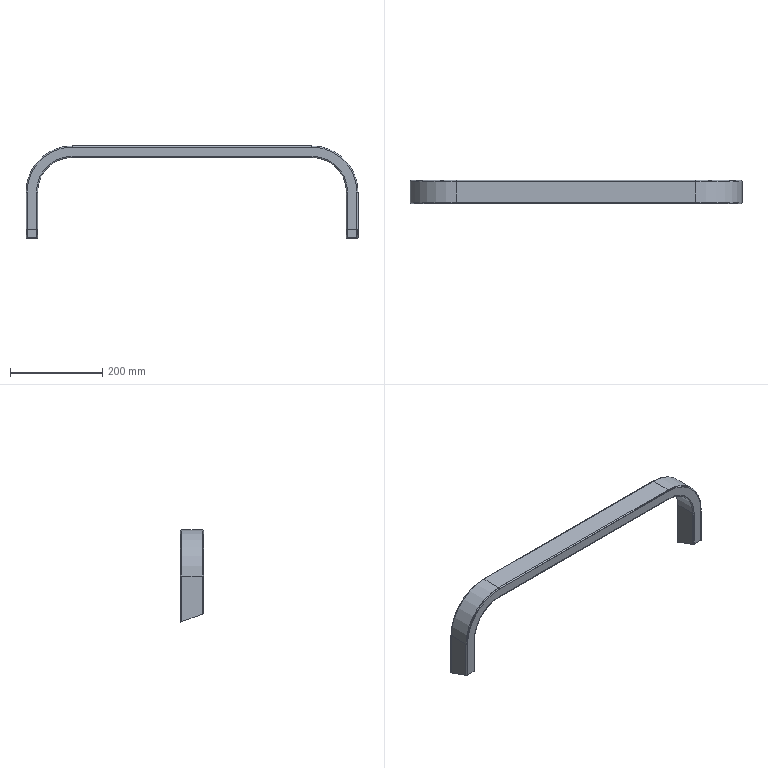Part | STEP file | 7471301 | 1 solid | 66 faces | box 720 x 50 x 200 mm | volume 206564 mm3 | cylinder 32 | plane 18 | torus 16 | commonest cylinder face diameters 2 x12 5 x12 150 x2 153 x2 197 x2 200 x2